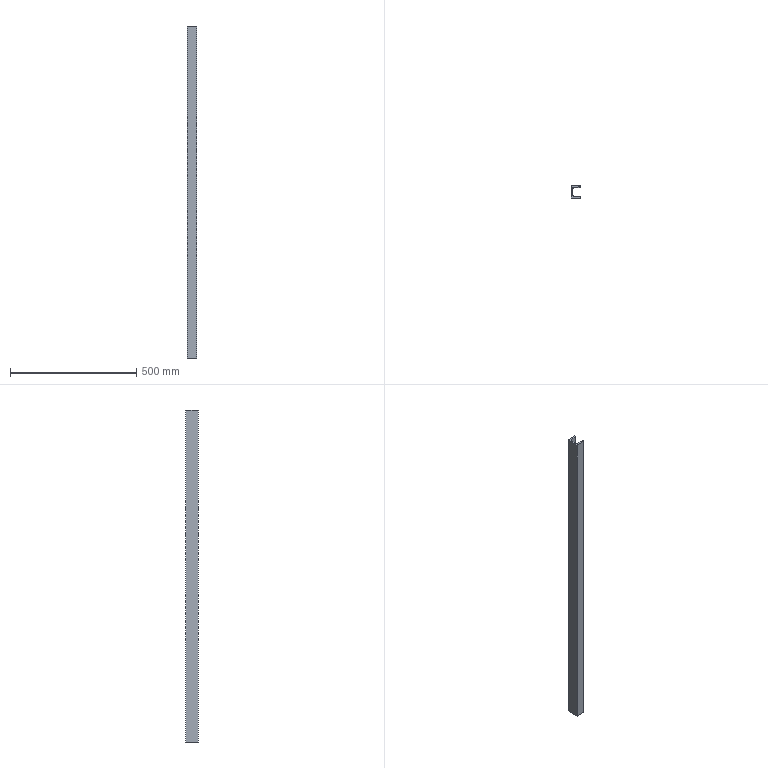Part | STEP file | DIN 1026-1 U 50 1785357045320 | 1 solid | 14 faces | box 38 x 50 x 1315 mm | volume 935965 mm3 | plane 10 | cylinder 4 | commonest cylinder face diameters 7 x2 14 x2
STEP:
#1=CARTESIAN_POINT('',(5.,-10.418,1314.813));
#2=VERTEX_POINT('',#1);
#3=CARTESIAN_POINT('',(11.442,-17.395,1314.813));
#4=VERTEX_POINT('',#3);
#5=CARTESIAN_POINT('',(12.,-10.418,1314.813));
#6=DIRECTION('',(0.,0.,1.));
#7=DIRECTION('',(-1.,0.,0.));
#8=AXIS2_PLACEMENT_3D('',#5,#6,#7);
#9=CIRCLE('',#8,7.);
#10=EDGE_CURVE('',#2,#4,#9,.T.);
#11=ORIENTED_EDGE('',*,*,#10,.T.);
#12=CARTESIAN_POINT('',(11.442,-17.395,0.));
#13=VERTEX_POINT('',#12);
#14=CARTESIAN_POINT('',(11.442,-17.395,0.));
#15=DIRECTION('',(0.,0.,1.));
#16=VECTOR('',#15,10.);
#17=LINE('',#14,#16);
#18=EDGE_CURVE('',#13,#4,#17,.T.);
#19=ORIENTED_EDGE('',*,*,#18,.F.);
#20=CARTESIAN_POINT('',(5.,-10.418,0.));
#21=VERTEX_POINT('',#20);
#22=CARTESIAN_POINT('',(12.,-10.418,0.));
#23=DIRECTION('',(0.,0.,1.));
#24=DIRECTION('',(-1.,0.,0.));
#25=AXIS2_PLACEMENT_3D('',#22,#23,#24);
#26=CIRCLE('',#25,7.);
#27=EDGE_CURVE('',#21,#13,#26,.T.);
#28=ORIENTED_EDGE('',*,*,#27,.F.);
#29=CARTESIAN_POINT('',(5.,-10.418,0.));
#30=DIRECTION('',(0.,0.,1.));
#31=VECTOR('',#30,10.);
#32=LINE('',#29,#31);
#33=EDGE_CURVE('',#21,#2,#32,.T.);
#34=ORIENTED_EDGE('',*,*,#33,.T.);
#35=EDGE_LOOP('',(#11,#19,#28,#34));
#36=FACE_OUTER_BOUND('',#35,.T.);
#37=CARTESIAN_POINT('',(12.,-10.418,0.));
#38=DIRECTION('',(0.,0.,1.));
#39=DIRECTION('',(-1.,0.,0.));
#40=AXIS2_PLACEMENT_3D('',#37,#38,#39);
#41=CYLINDRICAL_SURFACE('',#40,7.);
#42=ADVANCED_FACE('',(#36),#41,.F.);
#43=CARTESIAN_POINT('',(34.779,-19.262,1314.813));
#44=VERTEX_POINT('',#43);
#45=CARTESIAN_POINT('',(14.505,-17.64,1314.813));
#46=DIRECTION('',(0.9968,-0.07975,0.));
#47=VECTOR('',#46,10.);
#48=LINE('',#45,#47);
#49=EDGE_CURVE('',#4,#44,#48,.T.);
#50=ORIENTED_EDGE('',*,*,#49,.T.);
#51=CARTESIAN_POINT('',(34.779,-19.262,0.));
#52=VERTEX_POINT('',#51);
#53=CARTESIAN_POINT('',(34.779,-19.262,0.));
#54=DIRECTION('',(0.,0.,1.));
#55=VECTOR('',#54,10.);
#56=LINE('',#53,#55);
#57=EDGE_CURVE('',#52,#44,#56,.T.);
#58=ORIENTED_EDGE('',*,*,#57,.F.);
#59=CARTESIAN_POINT('',(14.505,-17.64,0.));
#60=DIRECTION('',(0.9968,-0.07975,0.));
#61=VECTOR('',#60,10.);
#62=LINE('',#59,#61);
#63=EDGE_CURVE('',#13,#52,#62,.T.);
#64=ORIENTED_EDGE('',*,*,#63,.F.);
#65=ORIENTED_EDGE('',*,*,#18,.T.);
#66=EDGE_LOOP('',(#50,#58,#64,#65));
#67=FACE_OUTER_BOUND('',#66,.T.);
#68=CARTESIAN_POINT('',(11.442,-17.395,0.));
#69=DIRECTION('',(0.07975,0.9968,0.));
#70=DIRECTION('',(0.,0.,1.));
#71=AXIS2_PLACEMENT_3D('',#68,#69,#70);
#72=PLANE('',#71);
#73=ADVANCED_FACE('',(#67),#72,.T.);
#74=CARTESIAN_POINT('',(38.,-22.751,1314.813));
#75=VERTEX_POINT('',#74);
#76=CARTESIAN_POINT('',(34.5,-22.751,1314.813));
#77=DIRECTION('',(0.,0.,-1.));
#78=DIRECTION('',(-1.,0.,0.));
#79=AXIS2_PLACEMENT_3D('',#76,#77,#78);
#80=CIRCLE('',#79,3.5);
#81=EDGE_CURVE('',#44,#75,#80,.T.);
#82=ORIENTED_EDGE('',*,*,#81,.T.);
#83=CARTESIAN_POINT('',(38.,-22.751,0.));
#84=VERTEX_POINT('',#83);
#85=CARTESIAN_POINT('',(38.,-22.751,0.));
#86=DIRECTION('',(0.,0.,1.));
#87=VECTOR('',#86,10.);
#88=LINE('',#85,#87);
#89=EDGE_CURVE('',#84,#75,#88,.T.);
#90=ORIENTED_EDGE('',*,*,#89,.F.);
#91=CARTESIAN_POINT('',(34.5,-22.751,0.));
#92=DIRECTION('',(0.,0.,-1.));
#93=DIRECTION('',(-1.,0.,0.));
#94=AXIS2_PLACEMENT_3D('',#91,#92,#93);
#95=CIRCLE('',#94,3.5);
#96=EDGE_CURVE('',#52,#84,#95,.T.);
#97=ORIENTED_EDGE('',*,*,#96,.F.);
#98=ORIENTED_EDGE('',*,*,#57,.T.);
#99=EDGE_LOOP('',(#82,#90,#97,#98));
#100=FACE_OUTER_BOUND('',#99,.T.);
#101=CARTESIAN_POINT('',(34.5,-22.751,0.));
#102=DIRECTION('',(0.,0.,1.));
#103=DIRECTION('',(-1.,0.,0.));
#104=AXIS2_PLACEMENT_3D('',#101,#102,#103);
#105=CYLINDRICAL_SURFACE('',#104,3.5);
#106=ADVANCED_FACE('',(#100),#105,.T.);
#107=CARTESIAN_POINT('',(38.,-25.,1314.813));
#108=VERTEX_POINT('',#107);
#109=CARTESIAN_POINT('',(38.,-11.376,1314.813));
#110=DIRECTION('',(0.,-1.,0.));
#111=VECTOR('',#110,10.);
#112=LINE('',#109,#111);
#113=EDGE_CURVE('',#75,#108,#112,.T.);
#114=ORIENTED_EDGE('',*,*,#113,.T.);
#115=CARTESIAN_POINT('',(38.,-25.,0.));
#116=VERTEX_POINT('',#115);
#117=CARTESIAN_POINT('',(38.,-25.,0.));
#118=DIRECTION('',(0.,0.,1.));
#119=VECTOR('',#118,10.);
#120=LINE('',#117,#119);
#121=EDGE_CURVE('',#116,#108,#120,.T.);
#122=ORIENTED_EDGE('',*,*,#121,.F.);
#123=CARTESIAN_POINT('',(38.,-11.376,0.));
#124=DIRECTION('',(0.,-1.,0.));
#125=VECTOR('',#124,10.);
#126=LINE('',#123,#125);
#127=EDGE_CURVE('',#84,#116,#126,.T.);
#128=ORIENTED_EDGE('',*,*,#127,.F.);
#129=ORIENTED_EDGE('',*,*,#89,.T.);
#130=EDGE_LOOP('',(#114,#122,#128,#129));
#131=FACE_OUTER_BOUND('',#130,.T.);
#132=CARTESIAN_POINT('',(38.,-22.751,0.));
#133=DIRECTION('',(1.,0.,0.));
#134=DIRECTION('',(0.,0.,-1.));
#135=AXIS2_PLACEMENT_3D('',#132,#133,#134);
#136=PLANE('',#135);
#137=ADVANCED_FACE('',(#131),#136,.T.);
#138=CARTESIAN_POINT('',(0.,-25.,1314.813));
#139=VERTEX_POINT('',#138);
#140=CARTESIAN_POINT('',(28.5,-25.,1314.813));
#141=DIRECTION('',(-1.,0.,0.));
#142=VECTOR('',#141,10.);
#143=LINE('',#140,#142);
#144=EDGE_CURVE('',#108,#139,#143,.T.);
#145=ORIENTED_EDGE('',*,*,#144,.T.);
#146=CARTESIAN_POINT('',(0.,-25.,0.));
#147=VERTEX_POINT('',#146);
#148=CARTESIAN_POINT('',(0.,-25.,0.));
#149=DIRECTION('',(0.,0.,1.));
#150=VECTOR('',#149,10.);
#151=LINE('',#148,#150);
#152=EDGE_CURVE('',#147,#139,#151,.T.);
#153=ORIENTED_EDGE('',*,*,#152,.F.);
#154=CARTESIAN_POINT('',(28.5,-25.,0.));
#155=DIRECTION('',(-1.,0.,0.));
#156=VECTOR('',#155,10.);
#157=LINE('',#154,#156);
#158=EDGE_CURVE('',#116,#147,#157,.T.);
#159=ORIENTED_EDGE('',*,*,#158,.F.);
#160=ORIENTED_EDGE('',*,*,#121,.T.);
#161=EDGE_LOOP('',(#145,#153,#159,#160));
#162=FACE_OUTER_BOUND('',#161,.T.);
#163=CARTESIAN_POINT('',(38.,-25.,0.));
#164=DIRECTION('',(0.,-1.,0.));
#165=DIRECTION('',(0.,0.,-1.));
#166=AXIS2_PLACEMENT_3D('',#163,#164,#165);
#167=PLANE('',#166);
#168=ADVANCED_FACE('',(#162),#167,.T.);
#169=CARTESIAN_POINT('',(0.,25.,1314.813));
#170=VERTEX_POINT('',#169);
#171=CARTESIAN_POINT('',(0.,0.,1314.813));
#172=DIRECTION('',(0.,1.,0.));
#173=VECTOR('',#172,10.);
#174=LINE('',#171,#173);
#175=EDGE_CURVE('',#139,#170,#174,.T.);
#176=ORIENTED_EDGE('',*,*,#175,.T.);
#177=CARTESIAN_POINT('',(0.,25.,0.));
#178=VERTEX_POINT('',#177);
#179=CARTESIAN_POINT('',(0.,25.,0.));
#180=DIRECTION('',(0.,0.,1.));
#181=VECTOR('',#180,10.);
#182=LINE('',#179,#181);
#183=EDGE_CURVE('',#178,#170,#182,.T.);
#184=ORIENTED_EDGE('',*,*,#183,.F.);
#185=CARTESIAN_POINT('',(0.,0.,0.));
#186=DIRECTION('',(0.,1.,0.));
#187=VECTOR('',#186,10.);
#188=LINE('',#185,#187);
#189=EDGE_CURVE('',#147,#178,#188,.T.);
#190=ORIENTED_EDGE('',*,*,#189,.F.);
#191=ORIENTED_EDGE('',*,*,#152,.T.);
#192=EDGE_LOOP('',(#176,#184,#190,#191));
#193=FACE_OUTER_BOUND('',#192,.T.);
#194=CARTESIAN_POINT('',(0.,0.,0.));
#195=DIRECTION('',(-1.,0.,0.));
#196=DIRECTION('',(0.,0.,1.));
#197=AXIS2_PLACEMENT_3D('',#194,#195,#196);
#198=PLANE('',#197);
#199=ADVANCED_FACE('',(#193),#198,.T.);
#200=CARTESIAN_POINT('',(38.,25.,1314.813));
#201=VERTEX_POINT('',#200);
#202=CARTESIAN_POINT('',(9.5,25.,1314.813));
#203=DIRECTION('',(1.,0.,0.));
#204=VECTOR('',#203,10.);
#205=LINE('',#202,#204);
#206=EDGE_CURVE('',#170,#201,#205,.T.);
#207=ORIENTED_EDGE('',*,*,#206,.T.);
#208=CARTESIAN_POINT('',(38.,25.,0.));
#209=VERTEX_POINT('',#208);
#210=CARTESIAN_POINT('',(38.,25.,0.));
#211=DIRECTION('',(0.,0.,1.));
#212=VECTOR('',#211,10.);
#213=LINE('',#210,#212);
#214=EDGE_CURVE('',#209,#201,#213,.T.);
#215=ORIENTED_EDGE('',*,*,#214,.F.);
#216=CARTESIAN_POINT('',(9.5,25.,0.));
#217=DIRECTION('',(1.,0.,0.));
#218=VECTOR('',#217,10.);
#219=LINE('',#216,#218);
#220=EDGE_CURVE('',#178,#209,#219,.T.);
#221=ORIENTED_EDGE('',*,*,#220,.F.);
#222=ORIENTED_EDGE('',*,*,#183,.T.);
#223=EDGE_LOOP('',(#207,#215,#221,#222));
#224=FACE_OUTER_BOUND('',#223,.T.);
#225=CARTESIAN_POINT('',(0.,25.,0.));
#226=DIRECTION('',(0.,1.,0.));
#227=DIRECTION('',(0.,0.,1.));
#228=AXIS2_PLACEMENT_3D('',#225,#226,#227);
#229=PLANE('',#228);
#230=ADVANCED_FACE('',(#224),#229,.T.);
#231=CARTESIAN_POINT('',(38.,22.751,1314.813));
#232=VERTEX_POINT('',#231);
#233=CARTESIAN_POINT('',(38.,12.5,1314.813));
#234=DIRECTION('',(0.,-1.,0.));
#235=VECTOR('',#234,10.);
#236=LINE('',#233,#235);
#237=EDGE_CURVE('',#201,#232,#236,.T.);
#238=ORIENTED_EDGE('',*,*,#237,.T.);
#239=CARTESIAN_POINT('',(38.,22.751,0.));
#240=VERTEX_POINT('',#239);
#241=CARTESIAN_POINT('',(38.,22.751,0.));
#242=DIRECTION('',(0.,0.,1.));
#243=VECTOR('',#242,10.);
#244=LINE('',#241,#243);
#245=EDGE_CURVE('',#240,#232,#244,.T.);
#246=ORIENTED_EDGE('',*,*,#245,.F.);
#247=CARTESIAN_POINT('',(38.,12.5,0.));
#248=DIRECTION('',(0.,-1.,0.));
#249=VECTOR('',#248,10.);
#250=LINE('',#247,#249);
#251=EDGE_CURVE('',#209,#240,#250,.T.);
#252=ORIENTED_EDGE('',*,*,#251,.F.);
#253=ORIENTED_EDGE('',*,*,#214,.T.);
#254=EDGE_LOOP('',(#238,#246,#252,#253));
#255=FACE_OUTER_BOUND('',#254,.T.);
#256=CARTESIAN_POINT('',(38.,25.,0.));
#257=DIRECTION('',(1.,0.,0.));
#258=DIRECTION('',(0.,0.,-1.));
#259=AXIS2_PLACEMENT_3D('',#256,#257,#258);
#260=PLANE('',#259);
#261=ADVANCED_FACE('',(#255),#260,.T.);
#262=CARTESIAN_POINT('',(34.779,19.262,1314.813));
#263=VERTEX_POINT('',#262);
#264=CARTESIAN_POINT('',(34.5,22.751,1314.813));
#265=DIRECTION('',(0.,0.,-1.));
#266=DIRECTION('',(-0.07975,0.9968,0.));
#267=AXIS2_PLACEMENT_3D('',#264,#265,#266);
#268=CIRCLE('',#267,3.5);
#269=EDGE_CURVE('',#232,#263,#268,.T.);
#270=ORIENTED_EDGE('',*,*,#269,.T.);
#271=CARTESIAN_POINT('',(34.779,19.262,0.));
#272=VERTEX_POINT('',#271);
#273=CARTESIAN_POINT('',(34.779,19.262,0.));
#274=DIRECTION('',(0.,0.,1.));
#275=VECTOR('',#274,10.);
#276=LINE('',#273,#275);
#277=EDGE_CURVE('',#272,#263,#276,.T.);
#278=ORIENTED_EDGE('',*,*,#277,.F.);
#279=CARTESIAN_POINT('',(34.5,22.751,0.));
#280=DIRECTION('',(0.,0.,-1.));
#281=DIRECTION('',(-0.07975,0.9968,0.));
#282=AXIS2_PLACEMENT_3D('',#279,#280,#281);
#283=CIRCLE('',#282,3.5);
#284=EDGE_CURVE('',#240,#272,#283,.T.);
#285=ORIENTED_EDGE('',*,*,#284,.F.);
#286=ORIENTED_EDGE('',*,*,#245,.T.);
#287=EDGE_LOOP('',(#270,#278,#285,#286));
#288=FACE_OUTER_BOUND('',#287,.T.);
#289=CARTESIAN_POINT('',(34.5,22.751,0.));
#290=DIRECTION('',(0.,0.,1.));
#291=DIRECTION('',(-0.07975,0.9968,0.));
#292=AXIS2_PLACEMENT_3D('',#289,#290,#291);
#293=CYLINDRICAL_SURFACE('',#292,3.5);
#294=ADVANCED_FACE('',(#288),#293,.T.);
#295=CARTESIAN_POINT('',(11.442,17.395,1314.813));
#296=VERTEX_POINT('',#295);
#297=CARTESIAN_POINT('',(26.174,18.574,1314.813));
#298=DIRECTION('',(-0.9968,-0.07975,0.));
#299=VECTOR('',#298,10.);
#300=LINE('',#297,#299);
#301=EDGE_CURVE('',#263,#296,#300,.T.);
#302=ORIENTED_EDGE('',*,*,#301,.T.);
#303=CARTESIAN_POINT('',(11.442,17.395,0.));
#304=VERTEX_POINT('',#303);
#305=CARTESIAN_POINT('',(11.442,17.395,0.));
#306=DIRECTION('',(0.,0.,1.));
#307=VECTOR('',#306,10.);
#308=LINE('',#305,#307);
#309=EDGE_CURVE('',#304,#296,#308,.T.);
#310=ORIENTED_EDGE('',*,*,#309,.F.);
#311=CARTESIAN_POINT('',(26.174,18.574,0.));
#312=DIRECTION('',(-0.9968,-0.07975,0.));
#313=VECTOR('',#312,10.);
#314=LINE('',#311,#313);
#315=EDGE_CURVE('',#272,#304,#314,.T.);
#316=ORIENTED_EDGE('',*,*,#315,.F.);
#317=ORIENTED_EDGE('',*,*,#277,.T.);
#318=EDGE_LOOP('',(#302,#310,#316,#317));
#319=FACE_OUTER_BOUND('',#318,.T.);
#320=CARTESIAN_POINT('',(34.779,19.262,0.));
#321=DIRECTION('',(0.07975,-0.9968,0.));
#322=DIRECTION('',(0.,0.,-1.));
#323=AXIS2_PLACEMENT_3D('',#320,#321,#322);
#324=PLANE('',#323);
#325=ADVANCED_FACE('',(#319),#324,.T.);
#326=CARTESIAN_POINT('',(5.,10.418,1314.813));
#327=VERTEX_POINT('',#326);
#328=CARTESIAN_POINT('',(12.,10.418,1314.813));
#329=DIRECTION('',(0.,0.,1.));
#330=DIRECTION('',(-0.07975,0.9968,0.));
#331=AXIS2_PLACEMENT_3D('',#328,#329,#330);
#332=CIRCLE('',#331,7.);
#333=EDGE_CURVE('',#296,#327,#332,.T.);
#334=ORIENTED_EDGE('',*,*,#333,.T.);
#335=CARTESIAN_POINT('',(5.,10.418,0.));
#336=VERTEX_POINT('',#335);
#337=CARTESIAN_POINT('',(5.,10.418,0.));
#338=DIRECTION('',(0.,0.,1.));
#339=VECTOR('',#338,10.);
#340=LINE('',#337,#339);
#341=EDGE_CURVE('',#336,#327,#340,.T.);
#342=ORIENTED_EDGE('',*,*,#341,.F.);
#343=CARTESIAN_POINT('',(12.,10.418,0.));
#344=DIRECTION('',(0.,0.,1.));
#345=DIRECTION('',(-0.07975,0.9968,0.));
#346=AXIS2_PLACEMENT_3D('',#343,#344,#345);
#347=CIRCLE('',#346,7.);
#348=EDGE_CURVE('',#304,#336,#347,.T.);
#349=ORIENTED_EDGE('',*,*,#348,.F.);
#350=ORIENTED_EDGE('',*,*,#309,.T.);
#351=EDGE_LOOP('',(#334,#342,#349,#350));
#352=FACE_OUTER_BOUND('',#351,.T.);
#353=CARTESIAN_POINT('',(12.,10.418,0.));
#354=DIRECTION('',(0.,0.,1.));
#355=DIRECTION('',(-0.07975,0.9968,0.));
#356=AXIS2_PLACEMENT_3D('',#353,#354,#355);
#357=CYLINDRICAL_SURFACE('',#356,7.);
#358=ADVANCED_FACE('',(#352),#357,.F.);
#359=CARTESIAN_POINT('',(5.,0.,1314.813));
#360=DIRECTION('',(0.,-1.,0.));
#361=VECTOR('',#360,10.);
#362=LINE('',#359,#361);
#363=EDGE_CURVE('',#327,#2,#362,.T.);
#364=ORIENTED_EDGE('',*,*,#363,.T.);
#365=ORIENTED_EDGE('',*,*,#33,.F.);
#366=CARTESIAN_POINT('',(5.,0.,0.));
#367=DIRECTION('',(0.,-1.,0.));
#368=VECTOR('',#367,10.);
#369=LINE('',#366,#368);
#370=EDGE_CURVE('',#336,#21,#369,.T.);
#371=ORIENTED_EDGE('',*,*,#370,.F.);
#372=ORIENTED_EDGE('',*,*,#341,.T.);
#373=EDGE_LOOP('',(#364,#365,#371,#372));
#374=FACE_OUTER_BOUND('',#373,.T.);
#375=CARTESIAN_POINT('',(5.,0.,0.));
#376=DIRECTION('',(1.,0.,0.));
#377=DIRECTION('',(0.,0.,-1.));
#378=AXIS2_PLACEMENT_3D('',#375,#376,#377);
#379=PLANE('',#378);
#380=ADVANCED_FACE('',(#374),#379,.T.);
#381=ORIENTED_EDGE('',*,*,#220,.T.);
#382=ORIENTED_EDGE('',*,*,#251,.T.);
#383=ORIENTED_EDGE('',*,*,#284,.T.);
#384=ORIENTED_EDGE('',*,*,#315,.T.);
#385=ORIENTED_EDGE('',*,*,#348,.T.);
#386=ORIENTED_EDGE('',*,*,#370,.T.);
#387=ORIENTED_EDGE('',*,*,#27,.T.);
#388=ORIENTED_EDGE('',*,*,#63,.T.);
#389=ORIENTED_EDGE('',*,*,#96,.T.);
#390=ORIENTED_EDGE('',*,*,#127,.T.);
#391=ORIENTED_EDGE('',*,*,#158,.T.);
#392=ORIENTED_EDGE('',*,*,#189,.T.);
#393=EDGE_LOOP('',(#381,#382,#383,#384,#385,#386,#387,#388,#389,#390,#391,#392));
#394=FACE_OUTER_BOUND('',#393,.T.);
#395=CARTESIAN_POINT('',(19.,0.,0.));
#396=DIRECTION('',(0.,0.,1.));
#397=DIRECTION('',(1.,0.,0.));
#398=AXIS2_PLACEMENT_3D('',#395,#396,#397);
#399=PLANE('',#398);
#400=ADVANCED_FACE('',(#394),#399,.F.);
#401=ORIENTED_EDGE('',*,*,#206,.F.);
#402=ORIENTED_EDGE('',*,*,#175,.F.);
#403=ORIENTED_EDGE('',*,*,#144,.F.);
#404=ORIENTED_EDGE('',*,*,#113,.F.);
#405=ORIENTED_EDGE('',*,*,#81,.F.);
#406=ORIENTED_EDGE('',*,*,#49,.F.);
#407=ORIENTED_EDGE('',*,*,#10,.F.);
#408=ORIENTED_EDGE('',*,*,#363,.F.);
#409=ORIENTED_EDGE('',*,*,#333,.F.);
#410=ORIENTED_EDGE('',*,*,#301,.F.);
#411=ORIENTED_EDGE('',*,*,#269,.F.);
#412=ORIENTED_EDGE('',*,*,#237,.F.);
#413=EDGE_LOOP('',(#401,#402,#403,#404,#405,#406,#407,#408,#409,#410,#411,#412));
#414=FACE_OUTER_BOUND('',#413,.T.);
#415=CARTESIAN_POINT('',(19.,0.,1314.813));
#416=DIRECTION('',(0.,0.,1.));
#417=DIRECTION('',(1.,0.,0.));
#418=AXIS2_PLACEMENT_3D('',#415,#416,#417);
#419=PLANE('',#418);
#420=ADVANCED_FACE('',(#414),#419,.T.);
#421=CLOSED_SHELL('',(#42,#73,#106,#137,#168,#199,#230,#261,#294,#325,#358,#380,#400,#420));
#422=MANIFOLD_SOLID_BREP('',#421);
#423=(LENGTH_UNIT()NAMED_UNIT(*)SI_UNIT(.MILLI.,.METRE.));
#424=UNCERTAINTY_MEASURE_WITH_UNIT(LENGTH_MEASURE(0.01),#423,'','');
#425=(NAMED_UNIT(*)PLANE_ANGLE_UNIT()SI_UNIT($,.RADIAN.));
#426=(NAMED_UNIT(*)SI_UNIT($,.STERADIAN.)SOLID_ANGLE_UNIT());
#427=(GEOMETRIC_REPRESENTATION_CONTEXT(3)GLOBAL_UNCERTAINTY_ASSIGNED_CONTEXT((#424))GLOBAL_UNIT_ASSIGNED_CONTEXT((#423,#425,#426))REPRESENTATION_CONTEXT('',''));
#428=ADVANCED_BREP_SHAPE_REPRESENTATION('',(#422),#427);